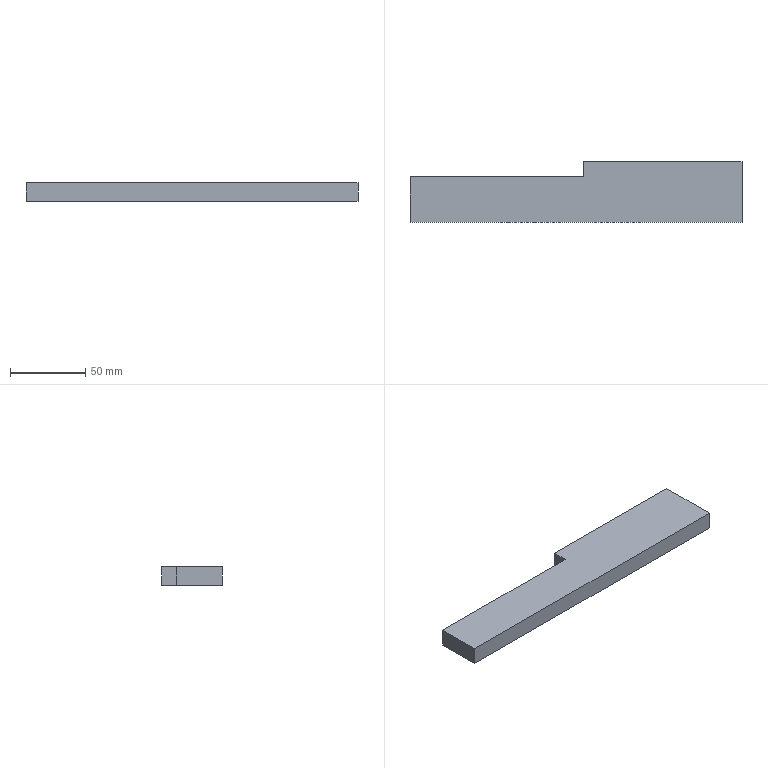Part | STEP file | 02-Square plate 1 | 1 solid | 8 faces | box 220 x 40 x 12 mm | volume 91800 mm3 | plane 8
STEP:
#1=CARTESIAN_POINT('',(0.,0.,0.));
#2=DIRECTION('',(0.,0.,1.));
#3=DIRECTION('',(1.,0.,0.));
#4=AXIS2_PLACEMENT_3D('',#1,#2,#3);
#5=CARTESIAN_POINT('',(0.,-40.,0.));
#6=VERTEX_POINT('',#5);
#7=CARTESIAN_POINT('',(0.,0.,0.));
#8=VERTEX_POINT('',#7);
#9=CARTESIAN_POINT('',(0.,0.,0.));
#10=DIRECTION('',(0.,1.,0.));
#11=VECTOR('',#10,1.);
#12=LINE('',#9,#11);
#13=CARTESIAN_POINT('',(0.,0.,12.));
#14=DIRECTION('',(-1.,0.,0.));
#15=DIRECTION('',(0.,-1.,0.));
#16=AXIS2_PLACEMENT_3D('',#13,#14,#15);
#17=PLANE('',#16);
#18=CARTESIAN_POINT('',(0.,-12.));
#19=DIRECTION('',(-1.,0.));
#20=VECTOR('',#19,1.);
#21=LINE('',#18,#20);
#22=(GEOMETRIC_REPRESENTATION_CONTEXT(2)PARAMETRIC_REPRESENTATION_CONTEXT()REPRESENTATION_CONTEXT('',''));
#23=DEFINITIONAL_REPRESENTATION('',(#21),#22);
#24=PCURVE('',#17,#23);
#25=CARTESIAN_POINT('',(0.,0.,0.));
#26=DIRECTION('',(0.,0.,-1.));
#27=DIRECTION('',(-1.,0.,0.));
#28=AXIS2_PLACEMENT_3D('',#25,#26,#27);
#29=PLANE('',#28);
#30=CARTESIAN_POINT('',(0.,0.));
#31=DIRECTION('',(0.,1.));
#32=VECTOR('',#31,1.);
#33=LINE('',#30,#32);
#34=(GEOMETRIC_REPRESENTATION_CONTEXT(2)PARAMETRIC_REPRESENTATION_CONTEXT()REPRESENTATION_CONTEXT('',''));
#35=DEFINITIONAL_REPRESENTATION('',(#33),#34);
#36=PCURVE('',#29,#35);
#37=SURFACE_CURVE('',#12,(#24,#36),.PCURVE_S1.);
#38=EDGE_CURVE('',#6,#8,#37,.T.);
#39=ORIENTED_EDGE('',*,*,#38,.T.);
#40=CARTESIAN_POINT('',(0.,0.,12.));
#41=VERTEX_POINT('',#40);
#42=CARTESIAN_POINT('',(0.,0.,12.));
#43=DIRECTION('',(0.,0.,-1.));
#44=VECTOR('',#43,1.);
#45=LINE('',#42,#44);
#46=CARTESIAN_POINT('',(0.,0.));
#47=DIRECTION('',(0.,-1.));
#48=VECTOR('',#47,1.);
#49=LINE('',#46,#48);
#50=(GEOMETRIC_REPRESENTATION_CONTEXT(2)PARAMETRIC_REPRESENTATION_CONTEXT()REPRESENTATION_CONTEXT('',''));
#51=DEFINITIONAL_REPRESENTATION('',(#49),#50);
#52=PCURVE('',#17,#51);
#53=CARTESIAN_POINT('',(0.,0.,12.));
#54=DIRECTION('',(0.,-1.,0.));
#55=DIRECTION('',(1.,0.,0.));
#56=AXIS2_PLACEMENT_3D('',#53,#54,#55);
#57=PLANE('',#56);
#58=CARTESIAN_POINT('',(0.,0.));
#59=DIRECTION('',(0.,-1.));
#60=VECTOR('',#59,1.);
#61=LINE('',#58,#60);
#62=(GEOMETRIC_REPRESENTATION_CONTEXT(2)PARAMETRIC_REPRESENTATION_CONTEXT()REPRESENTATION_CONTEXT('',''));
#63=DEFINITIONAL_REPRESENTATION('',(#61),#62);
#64=PCURVE('',#57,#63);
#65=SURFACE_CURVE('',#45,(#52,#64),.PCURVE_S1.);
#66=EDGE_CURVE('',#41,#8,#65,.T.);
#67=ORIENTED_EDGE('',*,*,#66,.F.);
#68=CARTESIAN_POINT('',(0.,-40.,12.));
#69=VERTEX_POINT('',#68);
#70=CARTESIAN_POINT('',(0.,0.,12.));
#71=DIRECTION('',(0.,1.,0.));
#72=VECTOR('',#71,1.);
#73=LINE('',#70,#72);
#74=CARTESIAN_POINT('',(0.,0.));
#75=DIRECTION('',(-1.,0.));
#76=VECTOR('',#75,1.);
#77=LINE('',#74,#76);
#78=(GEOMETRIC_REPRESENTATION_CONTEXT(2)PARAMETRIC_REPRESENTATION_CONTEXT()REPRESENTATION_CONTEXT('',''));
#79=DEFINITIONAL_REPRESENTATION('',(#77),#78);
#80=PCURVE('',#17,#79);
#81=CARTESIAN_POINT('',(0.,0.,12.));
#82=DIRECTION('',(0.,0.,-1.));
#83=DIRECTION('',(-1.,0.,0.));
#84=AXIS2_PLACEMENT_3D('',#81,#82,#83);
#85=PLANE('',#84);
#86=CARTESIAN_POINT('',(0.,0.));
#87=DIRECTION('',(0.,1.));
#88=VECTOR('',#87,1.);
#89=LINE('',#86,#88);
#90=(GEOMETRIC_REPRESENTATION_CONTEXT(2)PARAMETRIC_REPRESENTATION_CONTEXT()REPRESENTATION_CONTEXT('',''));
#91=DEFINITIONAL_REPRESENTATION('',(#89),#90);
#92=PCURVE('',#85,#91);
#93=SURFACE_CURVE('',#73,(#80,#92),.PCURVE_S1.);
#94=EDGE_CURVE('',#69,#41,#93,.T.);
#95=ORIENTED_EDGE('',*,*,#94,.F.);
#96=CARTESIAN_POINT('',(0.,-40.,12.));
#97=DIRECTION('',(0.,0.,-1.));
#98=VECTOR('',#97,1.);
#99=LINE('',#96,#98);
#100=CARTESIAN_POINT('',(40.,0.));
#101=DIRECTION('',(0.,-1.));
#102=VECTOR('',#101,1.);
#103=LINE('',#100,#102);
#104=(GEOMETRIC_REPRESENTATION_CONTEXT(2)PARAMETRIC_REPRESENTATION_CONTEXT()REPRESENTATION_CONTEXT('',''));
#105=DEFINITIONAL_REPRESENTATION('',(#103),#104);
#106=PCURVE('',#17,#105);
#107=CARTESIAN_POINT('',(0.,-40.,12.));
#108=DIRECTION('',(0.,1.,0.));
#109=DIRECTION('',(-1.,0.,0.));
#110=AXIS2_PLACEMENT_3D('',#107,#108,#109);
#111=PLANE('',#110);
#112=CARTESIAN_POINT('',(0.,0.));
#113=DIRECTION('',(0.,-1.));
#114=VECTOR('',#113,1.);
#115=LINE('',#112,#114);
#116=(GEOMETRIC_REPRESENTATION_CONTEXT(2)PARAMETRIC_REPRESENTATION_CONTEXT()REPRESENTATION_CONTEXT('',''));
#117=DEFINITIONAL_REPRESENTATION('',(#115),#116);
#118=PCURVE('',#111,#117);
#119=SURFACE_CURVE('',#99,(#106,#118),.PCURVE_S1.);
#120=EDGE_CURVE('',#69,#6,#119,.T.);
#121=ORIENTED_EDGE('',*,*,#120,.T.);
#122=EDGE_LOOP('',(#39,#67,#95,#121));
#123=FACE_BOUND('',#122,.T.);
#124=ADVANCED_FACE('',(#123),#17,.F.);
#125=CARTESIAN_POINT('',(-105.,0.,0.));
#126=VERTEX_POINT('',#125);
#127=CARTESIAN_POINT('',(0.,0.,0.));
#128=DIRECTION('',(-1.,0.,0.));
#129=VECTOR('',#128,1.);
#130=LINE('',#127,#129);
#131=CARTESIAN_POINT('',(0.,-12.));
#132=DIRECTION('',(-1.,0.));
#133=VECTOR('',#132,1.);
#134=LINE('',#131,#133);
#135=(GEOMETRIC_REPRESENTATION_CONTEXT(2)PARAMETRIC_REPRESENTATION_CONTEXT()REPRESENTATION_CONTEXT('',''));
#136=DEFINITIONAL_REPRESENTATION('',(#134),#135);
#137=PCURVE('',#57,#136);
#138=CARTESIAN_POINT('',(0.,0.));
#139=DIRECTION('',(1.,0.));
#140=VECTOR('',#139,1.);
#141=LINE('',#138,#140);
#142=(GEOMETRIC_REPRESENTATION_CONTEXT(2)PARAMETRIC_REPRESENTATION_CONTEXT()REPRESENTATION_CONTEXT('',''));
#143=DEFINITIONAL_REPRESENTATION('',(#141),#142);
#144=PCURVE('',#29,#143);
#145=SURFACE_CURVE('',#130,(#137,#144),.PCURVE_S1.);
#146=EDGE_CURVE('',#8,#126,#145,.T.);
#147=ORIENTED_EDGE('',*,*,#146,.T.);
#148=CARTESIAN_POINT('',(-105.,0.,12.));
#149=VERTEX_POINT('',#148);
#150=CARTESIAN_POINT('',(-105.,0.,12.));
#151=DIRECTION('',(0.,0.,-1.));
#152=VECTOR('',#151,1.);
#153=LINE('',#150,#152);
#154=CARTESIAN_POINT('',(-105.,0.));
#155=DIRECTION('',(0.,-1.));
#156=VECTOR('',#155,1.);
#157=LINE('',#154,#156);
#158=(GEOMETRIC_REPRESENTATION_CONTEXT(2)PARAMETRIC_REPRESENTATION_CONTEXT()REPRESENTATION_CONTEXT('',''));
#159=DEFINITIONAL_REPRESENTATION('',(#157),#158);
#160=PCURVE('',#57,#159);
#161=CARTESIAN_POINT('',(-105.,0.,12.));
#162=DIRECTION('',(1.,0.,0.));
#163=DIRECTION('',(0.,0.,-1.));
#164=AXIS2_PLACEMENT_3D('',#161,#162,#163);
#165=PLANE('',#164);
#166=CARTESIAN_POINT('',(0.,0.));
#167=DIRECTION('',(1.,0.));
#168=VECTOR('',#167,1.);
#169=LINE('',#166,#168);
#170=(GEOMETRIC_REPRESENTATION_CONTEXT(2)PARAMETRIC_REPRESENTATION_CONTEXT()REPRESENTATION_CONTEXT('',''));
#171=DEFINITIONAL_REPRESENTATION('',(#169),#170);
#172=PCURVE('',#165,#171);
#173=SURFACE_CURVE('',#153,(#160,#172),.PCURVE_S1.);
#174=EDGE_CURVE('',#149,#126,#173,.T.);
#175=ORIENTED_EDGE('',*,*,#174,.F.);
#176=CARTESIAN_POINT('',(0.,0.,12.));
#177=DIRECTION('',(-1.,0.,0.));
#178=VECTOR('',#177,1.);
#179=LINE('',#176,#178);
#180=CARTESIAN_POINT('',(0.,0.));
#181=DIRECTION('',(-1.,0.));
#182=VECTOR('',#181,1.);
#183=LINE('',#180,#182);
#184=(GEOMETRIC_REPRESENTATION_CONTEXT(2)PARAMETRIC_REPRESENTATION_CONTEXT()REPRESENTATION_CONTEXT('',''));
#185=DEFINITIONAL_REPRESENTATION('',(#183),#184);
#186=PCURVE('',#57,#185);
#187=CARTESIAN_POINT('',(0.,0.));
#188=DIRECTION('',(1.,0.));
#189=VECTOR('',#188,1.);
#190=LINE('',#187,#189);
#191=(GEOMETRIC_REPRESENTATION_CONTEXT(2)PARAMETRIC_REPRESENTATION_CONTEXT()REPRESENTATION_CONTEXT('',''));
#192=DEFINITIONAL_REPRESENTATION('',(#190),#191);
#193=PCURVE('',#85,#192);
#194=SURFACE_CURVE('',#179,(#186,#193),.PCURVE_S1.);
#195=EDGE_CURVE('',#41,#149,#194,.T.);
#196=ORIENTED_EDGE('',*,*,#195,.F.);
#197=ORIENTED_EDGE('',*,*,#66,.T.);
#198=EDGE_LOOP('',(#147,#175,#196,#197));
#199=FACE_BOUND('',#198,.T.);
#200=ADVANCED_FACE('',(#199),#57,.F.);
#201=CARTESIAN_POINT('',(-105.,-10.,0.));
#202=VERTEX_POINT('',#201);
#203=CARTESIAN_POINT('',(-105.,0.,0.));
#204=DIRECTION('',(0.,-1.,0.));
#205=VECTOR('',#204,1.);
#206=LINE('',#203,#205);
#207=CARTESIAN_POINT('',(12.,0.));
#208=DIRECTION('',(0.,-1.));
#209=VECTOR('',#208,1.);
#210=LINE('',#207,#209);
#211=(GEOMETRIC_REPRESENTATION_CONTEXT(2)PARAMETRIC_REPRESENTATION_CONTEXT()REPRESENTATION_CONTEXT('',''));
#212=DEFINITIONAL_REPRESENTATION('',(#210),#211);
#213=PCURVE('',#165,#212);
#214=CARTESIAN_POINT('',(105.,0.));
#215=DIRECTION('',(0.,-1.));
#216=VECTOR('',#215,1.);
#217=LINE('',#214,#216);
#218=(GEOMETRIC_REPRESENTATION_CONTEXT(2)PARAMETRIC_REPRESENTATION_CONTEXT()REPRESENTATION_CONTEXT('',''));
#219=DEFINITIONAL_REPRESENTATION('',(#217),#218);
#220=PCURVE('',#29,#219);
#221=SURFACE_CURVE('',#206,(#213,#220),.PCURVE_S1.);
#222=EDGE_CURVE('',#126,#202,#221,.T.);
#223=ORIENTED_EDGE('',*,*,#222,.T.);
#224=CARTESIAN_POINT('',(-105.,-10.,12.));
#225=VERTEX_POINT('',#224);
#226=CARTESIAN_POINT('',(-105.,-10.,12.));
#227=DIRECTION('',(0.,0.,-1.));
#228=VECTOR('',#227,1.);
#229=LINE('',#226,#228);
#230=CARTESIAN_POINT('',(0.,-10.));
#231=DIRECTION('',(1.,0.));
#232=VECTOR('',#231,1.);
#233=LINE('',#230,#232);
#234=(GEOMETRIC_REPRESENTATION_CONTEXT(2)PARAMETRIC_REPRESENTATION_CONTEXT()REPRESENTATION_CONTEXT('',''));
#235=DEFINITIONAL_REPRESENTATION('',(#233),#234);
#236=PCURVE('',#165,#235);
#237=CARTESIAN_POINT('',(-105.,-10.,12.));
#238=DIRECTION('',(0.,-1.,0.));
#239=DIRECTION('',(1.,0.,0.));
#240=AXIS2_PLACEMENT_3D('',#237,#238,#239);
#241=PLANE('',#240);
#242=CARTESIAN_POINT('',(0.,0.));
#243=DIRECTION('',(0.,-1.));
#244=VECTOR('',#243,1.);
#245=LINE('',#242,#244);
#246=(GEOMETRIC_REPRESENTATION_CONTEXT(2)PARAMETRIC_REPRESENTATION_CONTEXT()REPRESENTATION_CONTEXT('',''));
#247=DEFINITIONAL_REPRESENTATION('',(#245),#246);
#248=PCURVE('',#241,#247);
#249=SURFACE_CURVE('',#229,(#236,#248),.PCURVE_S1.);
#250=EDGE_CURVE('',#225,#202,#249,.T.);
#251=ORIENTED_EDGE('',*,*,#250,.F.);
#252=CARTESIAN_POINT('',(-105.,0.,12.));
#253=DIRECTION('',(0.,-1.,0.));
#254=VECTOR('',#253,1.);
#255=LINE('',#252,#254);
#256=CARTESIAN_POINT('',(0.,0.));
#257=DIRECTION('',(0.,-1.));
#258=VECTOR('',#257,1.);
#259=LINE('',#256,#258);
#260=(GEOMETRIC_REPRESENTATION_CONTEXT(2)PARAMETRIC_REPRESENTATION_CONTEXT()REPRESENTATION_CONTEXT('',''));
#261=DEFINITIONAL_REPRESENTATION('',(#259),#260);
#262=PCURVE('',#165,#261);
#263=CARTESIAN_POINT('',(105.,0.));
#264=DIRECTION('',(0.,-1.));
#265=VECTOR('',#264,1.);
#266=LINE('',#263,#265);
#267=(GEOMETRIC_REPRESENTATION_CONTEXT(2)PARAMETRIC_REPRESENTATION_CONTEXT()REPRESENTATION_CONTEXT('',''));
#268=DEFINITIONAL_REPRESENTATION('',(#266),#267);
#269=PCURVE('',#85,#268);
#270=SURFACE_CURVE('',#255,(#262,#269),.PCURVE_S1.);
#271=EDGE_CURVE('',#149,#225,#270,.T.);
#272=ORIENTED_EDGE('',*,*,#271,.F.);
#273=ORIENTED_EDGE('',*,*,#174,.T.);
#274=EDGE_LOOP('',(#223,#251,#272,#273));
#275=FACE_BOUND('',#274,.T.);
#276=ADVANCED_FACE('',(#275),#165,.F.);
#277=CARTESIAN_POINT('',(-220.,-10.,0.));
#278=VERTEX_POINT('',#277);
#279=CARTESIAN_POINT('',(-105.,-10.,0.));
#280=DIRECTION('',(-1.,0.,0.));
#281=VECTOR('',#280,1.);
#282=LINE('',#279,#281);
#283=CARTESIAN_POINT('',(0.,-12.));
#284=DIRECTION('',(-1.,0.));
#285=VECTOR('',#284,1.);
#286=LINE('',#283,#285);
#287=(GEOMETRIC_REPRESENTATION_CONTEXT(2)PARAMETRIC_REPRESENTATION_CONTEXT()REPRESENTATION_CONTEXT('',''));
#288=DEFINITIONAL_REPRESENTATION('',(#286),#287);
#289=PCURVE('',#241,#288);
#290=CARTESIAN_POINT('',(105.,-10.));
#291=DIRECTION('',(1.,0.));
#292=VECTOR('',#291,1.);
#293=LINE('',#290,#292);
#294=(GEOMETRIC_REPRESENTATION_CONTEXT(2)PARAMETRIC_REPRESENTATION_CONTEXT()REPRESENTATION_CONTEXT('',''));
#295=DEFINITIONAL_REPRESENTATION('',(#293),#294);
#296=PCURVE('',#29,#295);
#297=SURFACE_CURVE('',#282,(#289,#296),.PCURVE_S1.);
#298=EDGE_CURVE('',#202,#278,#297,.T.);
#299=ORIENTED_EDGE('',*,*,#298,.T.);
#300=CARTESIAN_POINT('',(-220.,-10.,12.));
#301=VERTEX_POINT('',#300);
#302=CARTESIAN_POINT('',(-220.,-10.,12.));
#303=DIRECTION('',(0.,0.,-1.));
#304=VECTOR('',#303,1.);
#305=LINE('',#302,#304);
#306=CARTESIAN_POINT('',(-115.,0.));
#307=DIRECTION('',(0.,-1.));
#308=VECTOR('',#307,1.);
#309=LINE('',#306,#308);
#310=(GEOMETRIC_REPRESENTATION_CONTEXT(2)PARAMETRIC_REPRESENTATION_CONTEXT()REPRESENTATION_CONTEXT('',''));
#311=DEFINITIONAL_REPRESENTATION('',(#309),#310);
#312=PCURVE('',#241,#311);
#313=CARTESIAN_POINT('',(-220.,-10.,12.));
#314=DIRECTION('',(1.,0.,0.));
#315=DIRECTION('',(0.,0.,-1.));
#316=AXIS2_PLACEMENT_3D('',#313,#314,#315);
#317=PLANE('',#316);
#318=CARTESIAN_POINT('',(0.,0.));
#319=DIRECTION('',(1.,0.));
#320=VECTOR('',#319,1.);
#321=LINE('',#318,#320);
#322=(GEOMETRIC_REPRESENTATION_CONTEXT(2)PARAMETRIC_REPRESENTATION_CONTEXT()REPRESENTATION_CONTEXT('',''));
#323=DEFINITIONAL_REPRESENTATION('',(#321),#322);
#324=PCURVE('',#317,#323);
#325=SURFACE_CURVE('',#305,(#312,#324),.PCURVE_S1.);
#326=EDGE_CURVE('',#301,#278,#325,.T.);
#327=ORIENTED_EDGE('',*,*,#326,.F.);
#328=CARTESIAN_POINT('',(-105.,-10.,12.));
#329=DIRECTION('',(-1.,0.,0.));
#330=VECTOR('',#329,1.);
#331=LINE('',#328,#330);
#332=CARTESIAN_POINT('',(0.,0.));
#333=DIRECTION('',(-1.,0.));
#334=VECTOR('',#333,1.);
#335=LINE('',#332,#334);
#336=(GEOMETRIC_REPRESENTATION_CONTEXT(2)PARAMETRIC_REPRESENTATION_CONTEXT()REPRESENTATION_CONTEXT('',''));
#337=DEFINITIONAL_REPRESENTATION('',(#335),#336);
#338=PCURVE('',#241,#337);
#339=CARTESIAN_POINT('',(105.,-10.));
#340=DIRECTION('',(1.,0.));
#341=VECTOR('',#340,1.);
#342=LINE('',#339,#341);
#343=(GEOMETRIC_REPRESENTATION_CONTEXT(2)PARAMETRIC_REPRESENTATION_CONTEXT()REPRESENTATION_CONTEXT('',''));
#344=DEFINITIONAL_REPRESENTATION('',(#342),#343);
#345=PCURVE('',#85,#344);
#346=SURFACE_CURVE('',#331,(#338,#345),.PCURVE_S1.);
#347=EDGE_CURVE('',#225,#301,#346,.T.);
#348=ORIENTED_EDGE('',*,*,#347,.F.);
#349=ORIENTED_EDGE('',*,*,#250,.T.);
#350=EDGE_LOOP('',(#299,#327,#348,#349));
#351=FACE_BOUND('',#350,.T.);
#352=ADVANCED_FACE('',(#351),#241,.F.);
#353=CARTESIAN_POINT('',(-220.,-40.,0.));
#354=VERTEX_POINT('',#353);
#355=CARTESIAN_POINT('',(-220.,-10.,0.));
#356=DIRECTION('',(0.,-1.,0.));
#357=VECTOR('',#356,1.);
#358=LINE('',#355,#357);
#359=CARTESIAN_POINT('',(12.,0.));
#360=DIRECTION('',(0.,-1.));
#361=VECTOR('',#360,1.);
#362=LINE('',#359,#361);
#363=(GEOMETRIC_REPRESENTATION_CONTEXT(2)PARAMETRIC_REPRESENTATION_CONTEXT()REPRESENTATION_CONTEXT('',''));
#364=DEFINITIONAL_REPRESENTATION('',(#362),#363);
#365=PCURVE('',#317,#364);
#366=CARTESIAN_POINT('',(220.,-10.));
#367=DIRECTION('',(0.,-1.));
#368=VECTOR('',#367,1.);
#369=LINE('',#366,#368);
#370=(GEOMETRIC_REPRESENTATION_CONTEXT(2)PARAMETRIC_REPRESENTATION_CONTEXT()REPRESENTATION_CONTEXT('',''));
#371=DEFINITIONAL_REPRESENTATION('',(#369),#370);
#372=PCURVE('',#29,#371);
#373=SURFACE_CURVE('',#358,(#365,#372),.PCURVE_S1.);
#374=EDGE_CURVE('',#278,#354,#373,.T.);
#375=ORIENTED_EDGE('',*,*,#374,.T.);
#376=CARTESIAN_POINT('',(-220.,-40.,12.));
#377=VERTEX_POINT('',#376);
#378=CARTESIAN_POINT('',(-220.,-40.,12.));
#379=DIRECTION('',(0.,0.,-1.));
#380=VECTOR('',#379,1.);
#381=LINE('',#378,#380);
#382=CARTESIAN_POINT('',(0.,-30.));
#383=DIRECTION('',(1.,0.));
#384=VECTOR('',#383,1.);
#385=LINE('',#382,#384);
#386=(GEOMETRIC_REPRESENTATION_CONTEXT(2)PARAMETRIC_REPRESENTATION_CONTEXT()REPRESENTATION_CONTEXT('',''));
#387=DEFINITIONAL_REPRESENTATION('',(#385),#386);
#388=PCURVE('',#317,#387);
#389=CARTESIAN_POINT('',(220.,0.));
#390=DIRECTION('',(0.,-1.));
#391=VECTOR('',#390,1.);
#392=LINE('',#389,#391);
#393=(GEOMETRIC_REPRESENTATION_CONTEXT(2)PARAMETRIC_REPRESENTATION_CONTEXT()REPRESENTATION_CONTEXT('',''));
#394=DEFINITIONAL_REPRESENTATION('',(#392),#393);
#395=PCURVE('',#111,#394);
#396=SURFACE_CURVE('',#381,(#388,#395),.PCURVE_S1.);
#397=EDGE_CURVE('',#377,#354,#396,.T.);
#398=ORIENTED_EDGE('',*,*,#397,.F.);
#399=CARTESIAN_POINT('',(-220.,-10.,12.));
#400=DIRECTION('',(0.,-1.,0.));
#401=VECTOR('',#400,1.);
#402=LINE('',#399,#401);
#403=CARTESIAN_POINT('',(0.,0.));
#404=DIRECTION('',(0.,-1.));
#405=VECTOR('',#404,1.);
#406=LINE('',#403,#405);
#407=(GEOMETRIC_REPRESENTATION_CONTEXT(2)PARAMETRIC_REPRESENTATION_CONTEXT()REPRESENTATION_CONTEXT('',''));
#408=DEFINITIONAL_REPRESENTATION('',(#406),#407);
#409=PCURVE('',#317,#408);
#410=CARTESIAN_POINT('',(220.,-10.));
#411=DIRECTION('',(0.,-1.));
#412=VECTOR('',#411,1.);
#413=LINE('',#410,#412);
#414=(GEOMETRIC_REPRESENTATION_CONTEXT(2)PARAMETRIC_REPRESENTATION_CONTEXT()REPRESENTATION_CONTEXT('',''));
#415=DEFINITIONAL_REPRESENTATION('',(#413),#414);
#416=PCURVE('',#85,#415);
#417=SURFACE_CURVE('',#402,(#409,#416),.PCURVE_S1.);
#418=EDGE_CURVE('',#301,#377,#417,.T.);
#419=ORIENTED_EDGE('',*,*,#418,.F.);
#420=ORIENTED_EDGE('',*,*,#326,.T.);
#421=EDGE_LOOP('',(#375,#398,#419,#420));
#422=FACE_BOUND('',#421,.T.);
#423=ADVANCED_FACE('',(#422),#317,.F.);
#424=CARTESIAN_POINT('',(0.,-40.,0.));
#425=DIRECTION('',(1.,0.,0.));
#426=VECTOR('',#425,1.);
#427=LINE('',#424,#426);
#428=CARTESIAN_POINT('',(0.,-12.));
#429=DIRECTION('',(-1.,0.));
#430=VECTOR('',#429,1.);
#431=LINE('',#428,#430);
#432=(GEOMETRIC_REPRESENTATION_CONTEXT(2)PARAMETRIC_REPRESENTATION_CONTEXT()REPRESENTATION_CONTEXT('',''));
#433=DEFINITIONAL_REPRESENTATION('',(#431),#432);
#434=PCURVE('',#111,#433);
#435=CARTESIAN_POINT('',(0.,-40.));
#436=DIRECTION('',(-1.,0.));
#437=VECTOR('',#436,1.);
#438=LINE('',#435,#437);
#439=(GEOMETRIC_REPRESENTATION_CONTEXT(2)PARAMETRIC_REPRESENTATION_CONTEXT()REPRESENTATION_CONTEXT('',''));
#440=DEFINITIONAL_REPRESENTATION('',(#438),#439);
#441=PCURVE('',#29,#440);
#442=SURFACE_CURVE('',#427,(#434,#441),.PCURVE_S1.);
#443=EDGE_CURVE('',#354,#6,#442,.T.);
#444=ORIENTED_EDGE('',*,*,#443,.T.);
#445=ORIENTED_EDGE('',*,*,#120,.F.);
#446=CARTESIAN_POINT('',(0.,-40.,12.));
#447=DIRECTION('',(1.,0.,0.));
#448=VECTOR('',#447,1.);
#449=LINE('',#446,#448);
#450=CARTESIAN_POINT('',(0.,0.));
#451=DIRECTION('',(-1.,0.));
#452=VECTOR('',#451,1.);
#453=LINE('',#450,#452);
#454=(GEOMETRIC_REPRESENTATION_CONTEXT(2)PARAMETRIC_REPRESENTATION_CONTEXT()REPRESENTATION_CONTEXT('',''));
#455=DEFINITIONAL_REPRESENTATION('',(#453),#454);
#456=PCURVE('',#111,#455);
#457=CARTESIAN_POINT('',(0.,-40.));
#458=DIRECTION('',(-1.,0.));
#459=VECTOR('',#458,1.);
#460=LINE('',#457,#459);
#461=(GEOMETRIC_REPRESENTATION_CONTEXT(2)PARAMETRIC_REPRESENTATION_CONTEXT()REPRESENTATION_CONTEXT('',''));
#462=DEFINITIONAL_REPRESENTATION('',(#460),#461);
#463=PCURVE('',#85,#462);
#464=SURFACE_CURVE('',#449,(#456,#463),.PCURVE_S1.);
#465=EDGE_CURVE('',#377,#69,#464,.T.);
#466=ORIENTED_EDGE('',*,*,#465,.F.);
#467=ORIENTED_EDGE('',*,*,#397,.T.);
#468=EDGE_LOOP('',(#444,#445,#466,#467));
#469=FACE_BOUND('',#468,.T.);
#470=ADVANCED_FACE('',(#469),#111,.F.);
#471=ORIENTED_EDGE('',*,*,#94,.T.);
#472=ORIENTED_EDGE('',*,*,#195,.T.);
#473=ORIENTED_EDGE('',*,*,#271,.T.);
#474=ORIENTED_EDGE('',*,*,#347,.T.);
#475=ORIENTED_EDGE('',*,*,#418,.T.);
#476=ORIENTED_EDGE('',*,*,#465,.T.);
#477=EDGE_LOOP('',(#471,#472,#473,#474,#475,#476));
#478=FACE_BOUND('',#477,.T.);
#479=ADVANCED_FACE('',(#478),#85,.F.);
#480=ORIENTED_EDGE('',*,*,#38,.F.);
#481=ORIENTED_EDGE('',*,*,#443,.F.);
#482=ORIENTED_EDGE('',*,*,#374,.F.);
#483=ORIENTED_EDGE('',*,*,#298,.F.);
#484=ORIENTED_EDGE('',*,*,#222,.F.);
#485=ORIENTED_EDGE('',*,*,#146,.F.);
#486=EDGE_LOOP('',(#480,#481,#482,#483,#484,#485));
#487=FACE_BOUND('',#486,.T.);
#488=ADVANCED_FACE('',(#487),#29,.T.);
#489=CLOSED_SHELL('',(#124,#200,#276,#352,#423,#470,#479,#488));
#490=MANIFOLD_SOLID_BREP('',#489);
#491=(LENGTH_UNIT()NAMED_UNIT(*)SI_UNIT(.MILLI.,.METRE.));
#492=UNCERTAINTY_MEASURE_WITH_UNIT(LENGTH_MEASURE(0.0000001),#491,'','');
#493=(NAMED_UNIT(*)PLANE_ANGLE_UNIT()SI_UNIT($,.RADIAN.));
#494=(NAMED_UNIT(*)SI_UNIT($,.STERADIAN.)SOLID_ANGLE_UNIT());
#495=(GEOMETRIC_REPRESENTATION_CONTEXT(3)GLOBAL_UNCERTAINTY_ASSIGNED_CONTEXT((#492))GLOBAL_UNIT_ASSIGNED_CONTEXT((#491,#493,#494))REPRESENTATION_CONTEXT('',''));
#496=ADVANCED_BREP_SHAPE_REPRESENTATION('',(#4,#490),#495);